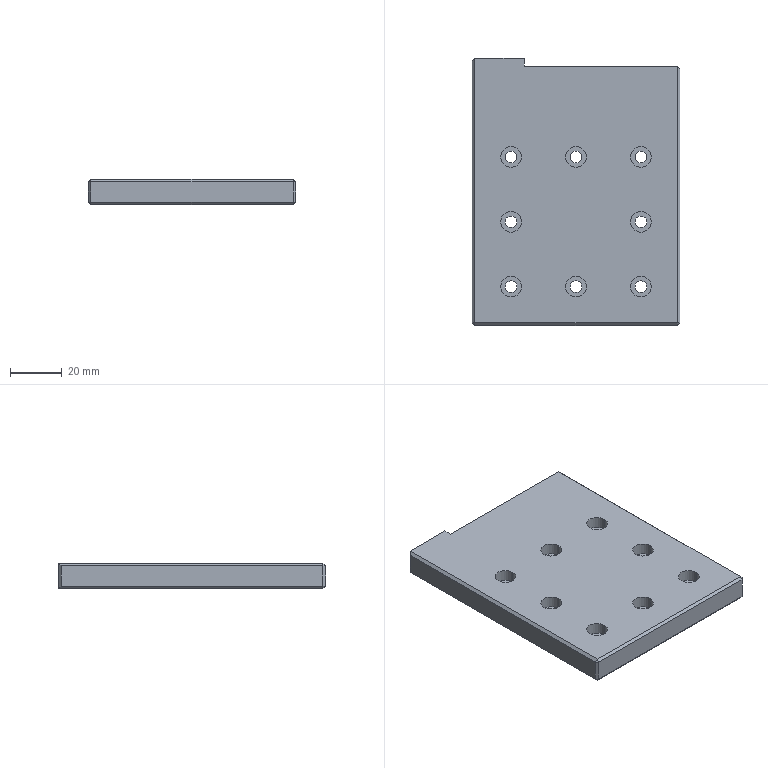Part | STEP file | MT-COMBO-119-S041 | 1 solid | 74 faces | box 80 x 103 x 10 mm | volume 77497 mm3 | cylinder 38 | plane 30 | cone 6 | commonest cylinder face diameters 4.5 x16 8 x16 3.3 x6